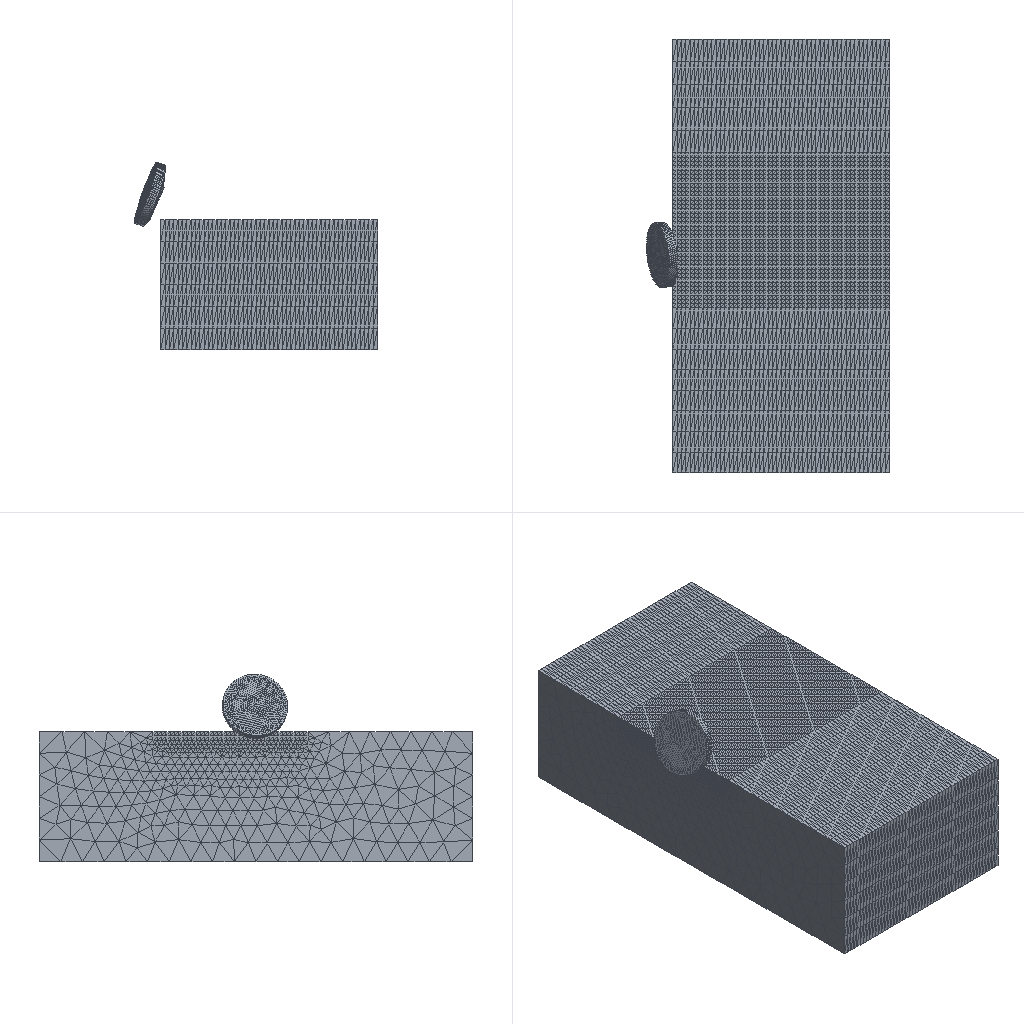Simulation study | abaqus
Set-up summary:
category,name,step,type,value,unit,region
solver,abaqus,,Abaqus/CAE 2024
units,mm-N-s-tonne (MPa),,inferred,E=890000 density=3.54e-09
analysis,Step-1,,dynamic explicit,nlgeom=True; time_period=0.06
mesh,nodes,,,20476
mesh,elements,,,102379
element_type,C3D4T,,,102379
material,tool-PDC,,E,890000
material,tool-PDC,,nu,0.077
material,tool-PDC,,density,3.54e-09
material,tool-PDC,,conductivity,543
material,tool-PDC,,specific_heat,7.9e+08
material,tool-PDC,,behaviors,conductivity; specific heat
material,tool-yingzhihejin,,E,570000
material,tool-yingzhihejin,,nu,0.22
material,tool-yingzhihejin,,density,1.5e-08
material,tool-yingzhihejin,,conductivity,110
material,tool-yingzhihejin,,specific_heat,2.03e+08
material,tool-yingzhihejin,,behaviors,conductivity; specific heat
material,work,,E,40000
material,work,,nu,0.25
material,work,,density,2.65e-09
material,work,,conductivity,3.5
material,work,,specific_heat,7.9e+08
material,work,,behaviors,plastic; conductivity; damage initiation; damage evolution; drucker prager; drucker prager hardening; specific heat
section,tool-PDC,,solid section,,,Set-1
section,work,,solid section,,,Set-15
load,Predefined,initial,initial condition temperature
load,workT,initial,initial condition temperature
bc,BC-1,initial,encastre,[dofs=ENCASTRE],,Set-4
bc,BC-2,Step-1,velocity,"1000 [dofs=rx,ry,rz,x,y,z n=6]",,Set-9
contact,Int-1,Step-1,contact pair,interaction=IntProp-1; friction=0.3; behavior=hard,,tool1.bztoolsurf / work_chipchipaaaaa_CNS_
constraint,rigid body,,,1
Abaqus input file, long lists of numbers shortened:
*Heading
** Job name: deck Model name: Model-1
** Generated by: Abaqus/CAE 2024
*Preprint, echo=NO, model=NO, history=NO, contact=NO
**
** PARTS
**
*Part, name=tool1
*Node
      1,           5.,  -2.887,           3.
      2,         3.75, -0.7217,           3.
** (5929 more lines like these left out)
*Element, type=C3D4T
    1, 2058, 2059, 2060, 2061
    2, 2058, 2059, 2061, 2062
** (29402 more lines like these left out)
*Nset, nset=Set-1, generate
    1,  5931,     1
*Elset, elset=Set-1, generate
     1,  29404,      1
*Elset, elset=bzrigid, generate
     1,  29404,      1
*Nset, nset=bztool-T, generate
    1,  5931,     1
*Elset, elset=_bztoolsurf_S1, internal
    34,  1298,  2256,  2732,  3026,  3216,  6503,  6610,  7632,  7763,  7802,  7903,  7919,  7999,  8086,  8121
  8182,  8228,  8234,  8236,  8258,  8504,  8597,  8762,  8786,  8792,  8829,  8902,  8924,  8983,  9014,  9018
** (6 more lines like these left out)
*Elset, elset=_bztoolsurf_S2, internal
   149,  1985,  2225,  2256,  2556,  2621,  2754,  2761,  2876,  2909,  2933,  2943,  3042,  3217,  3229,  3366
  3386,  3442,  3456,  3496,  3499,  3692,  3764,  3770,  3778,  3785,  3790,  3827,  3835,  3921,  3925,  4008
** (10 more lines like these left out)
*Elset, elset=_bztoolsurf_S3, internal
    29,    35,    54,    91,    98,   111,   126,   128,   131,   133,   158,   168,   183,   228,   258,   272
   291,   348,   396,   452,   461,   588,   609,   723,   813,   917,   920,   951,  1019,  1035,  1037,  1069
** (221 more lines like these left out)
*Elset, elset=_bztoolsurf_S4, internal
   173,   176,  1811,  2306,  2701,  2809,  2899,  3051,  3147,  3318,  3363,  3367,  3379,  3452,  3464,  3465
  3580,  3694,  3697,  3797,  3805,  3834,  3959,  4023,  4053,  4059,  4162,  4364,  4396,  4468,  4526,  4692
** (13 more lines like these left out)
*Surface, type=ELEMENT, name=bztoolsurf
_bztoolsurf_S1, S1
_bztoolsurf_S2, S2
_bztoolsurf_S4, S4
_bztoolsurf_S3, S3
** Section: tool2
*Solid Section, elset=Set-1, material=tool-PDC
,
*End Part
**
*Part, name=work
*Node
      1,          50.,  -26.243,          28.
      2,          50.,         -62.,          28.
** (14542 more lines like these left out)
*Element, type=C3D4T
    1,  4972,  4973,  4974,  4975
    2,  4972,  4976,  4977,  4978
** (72973 more lines like these left out)
*Nset, nset=Set-15, generate
     1,  14544,      1
*Elset, elset=Set-15, generate
     1,  72975,      1
*Nset, nset=workwenduchang, generate
     1,  14544,      1
*Nset, nset=chipchipaaaaa
     1,     2,     3,     8,     9,    14,    15,    16,    17,    18,    19,    20,    21,    22,    23,    24
    25,    26,    27,    28,    29,    30,    31,    32,    33,    34,    35,    36,    37,    38,    39,    40
** (429 more lines like these left out)
** Section: Section-1
*Solid Section, elset=Set-15, material=work
,
*End Part
**
**
** ASSEMBLY
**
*Assembly, name=Assembly
**
*Instance, name=work, part=work
-3.613, 40.291, 29.28
*End Instance
**
*Instance, name=tool1, part=tool1
-7.013, -9.581, 65.456
-7.013, -9.581, 65.456, -6.773, -8.641, 65.7, 115.002
*End Instance
**
*Node
      1,  -7.013,  -9.581,   65.456
*Nset, nset=Set-4, instance=work
    5,    6,   11,   12,   65,   66,   67,   68,   69,   70,   71,   72,   73,   74,   75,   76
   77,   78,   79,   80,   81,   82,   83,  234,  235,  236,  237,  238,  239,  240,  241,  242
** (65 more lines like these left out)
*Elset, elset=Set-4, instance=work
    32,   101,   228,   331,   408,   505,  1083,  1289,  1332,  2379,  2517,  2623,  2714,  3193,  3301,  3311
  3410,  3536,  3543,  3819,  5110,  5709,  6245,  6581,  6586,  6587,  6588,  6611,  6665,  6667,  6671,  6679
** (123 more lines like these left out)
*Nset, nset=Set-9
 1,
*Nset, nset=_PickedSet33, internal
 1,
*Surface, type=NODE, name=work_chipchipaaaaa_CNS_, internal
work.chipchipaaaaa, 1.
** Constraint: Constraint-1
*Rigid Body, ref node=_PickedSet33, elset=tool1.bzrigid
*End Assembly
**
** MATERIALS
**
*Material, name=tool-PDC
*Conductivity
543.,
*Density
 3.54e-09,
*Elastic
890000., 0.077
*Specific Heat
 7.9e+08,
*Material, name=tool-yingzhihejin
*Conductivity
110.,
*Density
 1.5e-08,
*Elastic
570000., 0.22
*Specific Heat
 2.03e+08,
*Material, name=work
*Conductivity
 3.5,
*Damage Initiation, criterion=JOHNSON COOK
 0.02,  0.38, -0.46,    0.,    0., 2000.,   20.,    1.
*Damage Evolution, type=DISPLACEMENT
 0.0002,
*Density
 2.65e-09,
*Drucker Prager
39., 0.95,  15.
*Drucker Prager Hardening, type=SHEAR
100.,0.
*Elastic
40000., 0.25
*Specific Heat
 7.9e+08,
**
** INTERACTION PROPERTIES
**
*Surface Interaction, name=IntProp-1
*Friction
 0.3,
*Surface Behavior, pressure-overclosure=HARD
**
** BOUNDARY CONDITIONS
**
** Name: BC-1 Type: Symmetry/Antisymmetry/Encastre
*Boundary
Set-4, ENCASTRE
**
** PREDEFINED FIELDS
**
** Name: Predefined Field-2   Type: Temperature
*Initial Conditions, type=TEMPERATURE
tool1.bztool-T, 25.
** Name: workT   Type: Temperature
*Initial Conditions, type=TEMPERATURE
work.workwenduchang, 25.
** ----------------------------------------------------------------
**
** STEP: Step-1
**
*Step, name=Step-1, nlgeom=YES
*Dynamic, Explicit
, 0.06
*Bulk Viscosity
0.06, 1.2
** Mass Scaling: Semi-Automatic
**               Whole Model
*Fixed Mass Scaling, factor=200.
**
** BOUNDARY CONDITIONS
**
** Name: BC-2 Type: Velocity/Angular velocity
*Boundary, type=VELOCITY
Set-9, 1, 1, 1000.
Set-9, 2, 2
Set-9, 3, 3
Set-9, 4, 4
Set-9, 5, 5
Set-9, 6, 6
**
** INTERACTIONS
**
** Interaction: Int-1
*Contact Pair, interaction=IntProp-1, mechanical constraint=KINEMATIC, cpset=Int-1
tool1.bztoolsurf, work_chipchipaaaaa_CNS_
**
** OUTPUT REQUESTS
**
*Restart, write, number interval=1, time marks=NO
**
** FIELD OUTPUT: F-Output-1
**
*Output, field, number interval=200
*Node Output
RT, U
*Element Output, directions=YES
MISES, PEEQ, STATUS, TEMP
**
** HISTORY OUTPUT: H-Output-1
**
*Output, history
*Energy Output
ALLAE, ALLCD, ALLCW, ALLDC, ALLDMD, ALLFD, ALLIE, ALLKE, ALLMW, ALLPD, ALLPW, ALLSE, ALLVD, ALLWK, ETOTAL
*End Step
Results summary:
result,odb.job_status,,,JOB_STATUS_COMPLETED_SUCCESSFULLY,"consistent, unstated (Abaqus has no unit system)"
result,steps[0].procedure,Step-1,,"*DYNAMIC, EXPLICIT","consistent, unstated (Abaqus has no unit system)"
result,steps[0].time_period,Step-1,,0.06,"consistent, unstated (Abaqus has no unit system)"
result,steps[0].n_frames,Step-1,,201,"consistent, unstated (Abaqus has no unit system)"
result,steps[0].last_frame.id,Step-1,,180192,"consistent, unstated (Abaqus has no unit system)"
result,steps[0].last_frame.value,Step-1,,0.06,"consistent, unstated (Abaqus has no unit system)"
result,steps[0].last_frame.description,Step-1,,Increment    180192: Step Time =   6.0000E-02,"consistent, unstated (Abaqus has no unit system)"
result,steps[0].completed,Step-1,,True,"consistent, unstated (Abaqus has no unit system)"
result,steps[0].max_U_magnitude,Step-1,,347.744,"consistent, unstated (Abaqus has no unit system)"
result,steps[0].max_S_mises,Step-1,,669.418,"consistent, unstated (Abaqus has no unit system)"
result,steps[0].diagnostic.n_increments,Step-1,,201,"consistent, unstated (Abaqus has no unit system)"